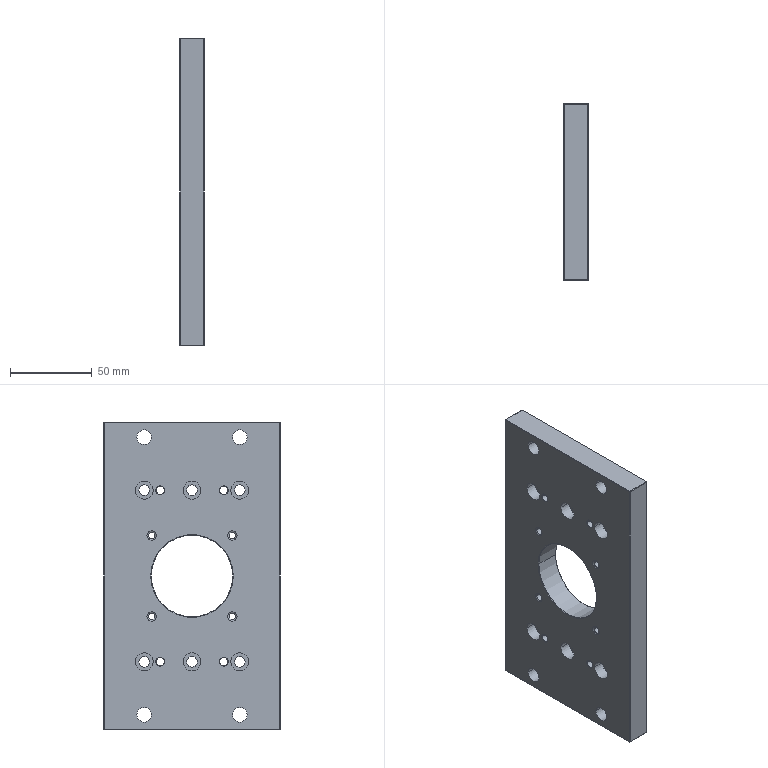Part | NX | 1 solid | 102 faces | box 15 x 108 x 188 mm | volume 263799 mm3 | cylinder 50 | cone 28 | plane 24 | commonest cylinder face diameters 6.5 x12 11 x12 4.2 x8 5 x8 9 x8 50 x2